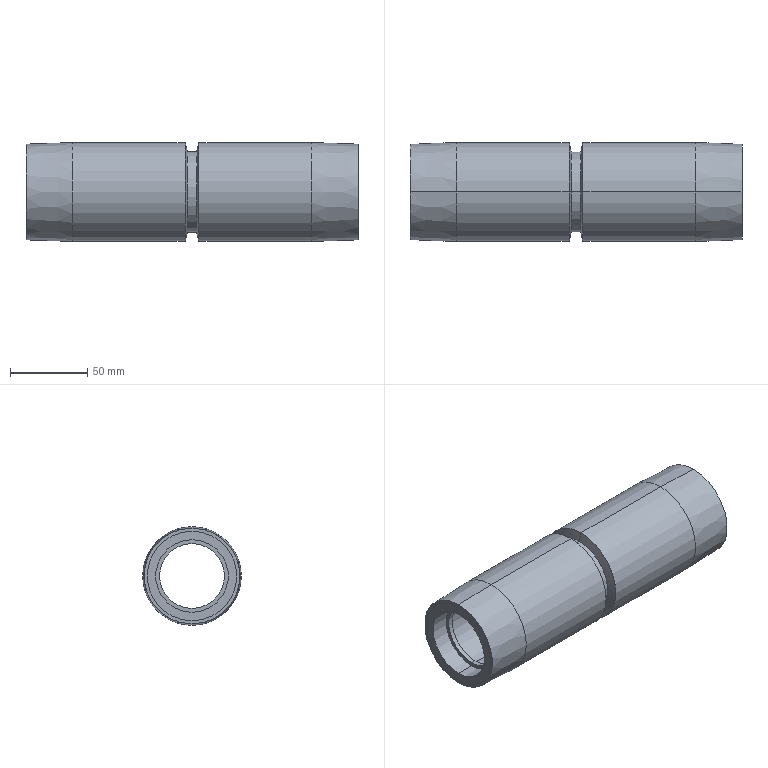Part | STEP file | MM-P46715-04_1 | 3 solids | 42 faces | box 215 x 64 x 64 mm | volume 333247 mm3 | cylinder 24 | plane 10 | cone 8 | commonest cylinder face diameters 58 x8 42 x4 47 x4 64 x4 45 x2 52 x2